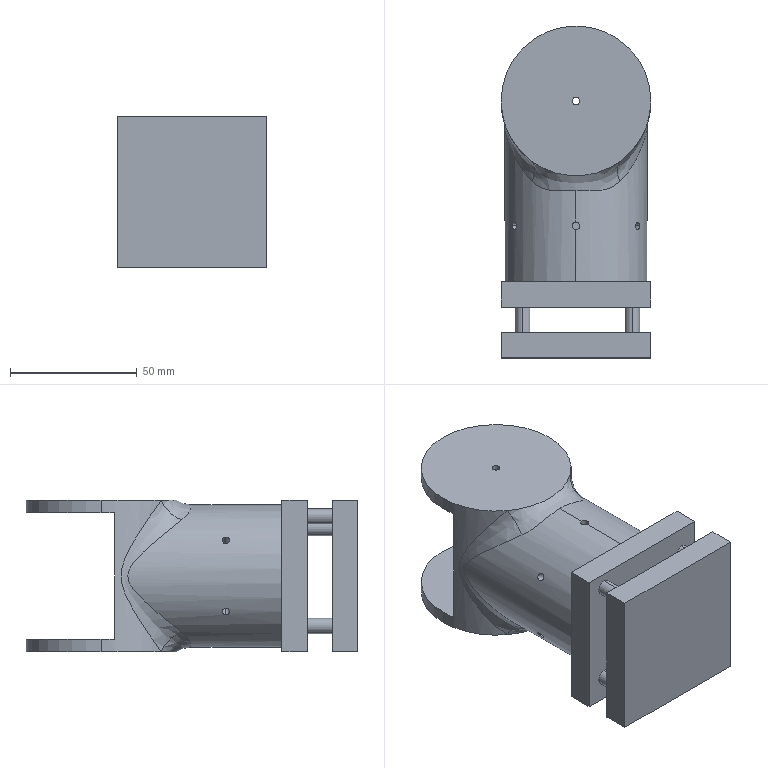Part | SolidWorks | features ICE 5, CirPattern 1, CutThin 1, Extrusion 1, Fillet 1 | 1 solid | 57 faces | box 59.155 x 131.009 x 60 mm | volume 266464 mm3 | cylinder 30 | plane 23 | spline 4 | commonest cylinder face diameters 3 x16 6 x8 59.155 x4 56.268 x2